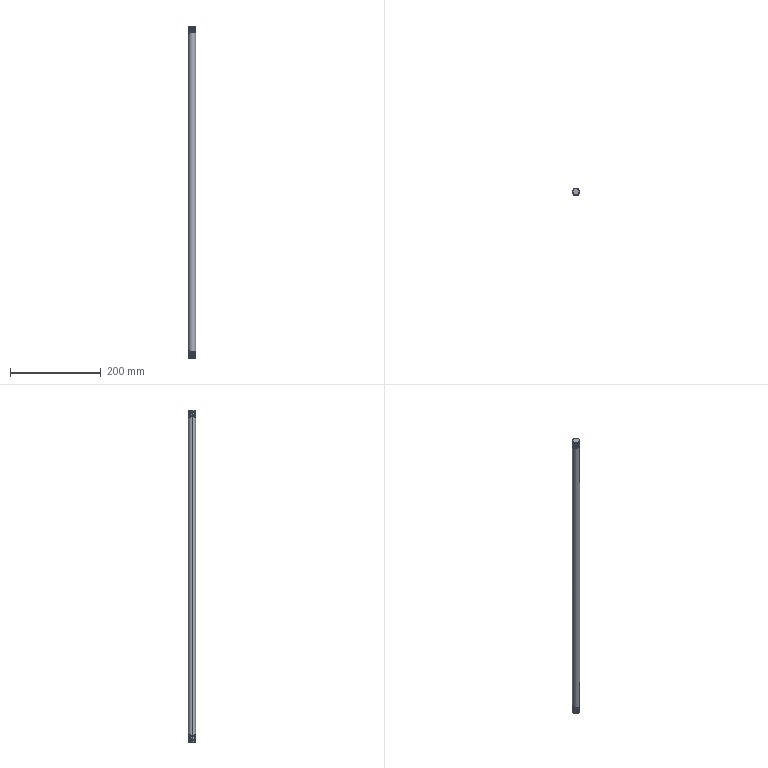Part | SolidWorks | features Extrusion 1, MirrorPattern 1, SweepThread 1 | 1 solid | 44 faces | box 16 x 16 x 730 mm | volume 145986 mm3 | cylinder 32 | plane 6 | spline 6 | commonest cylinder face diameters 16 x32